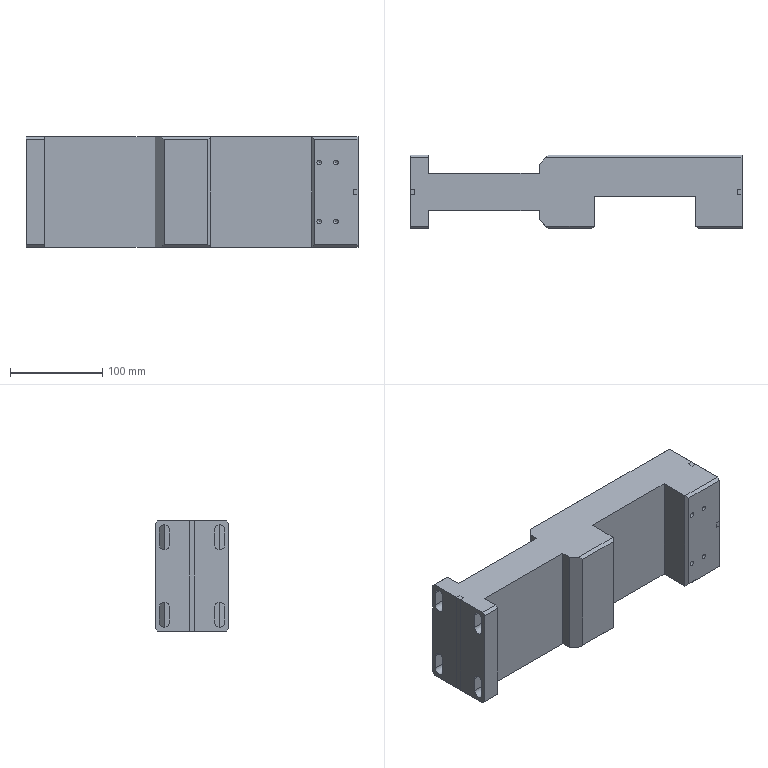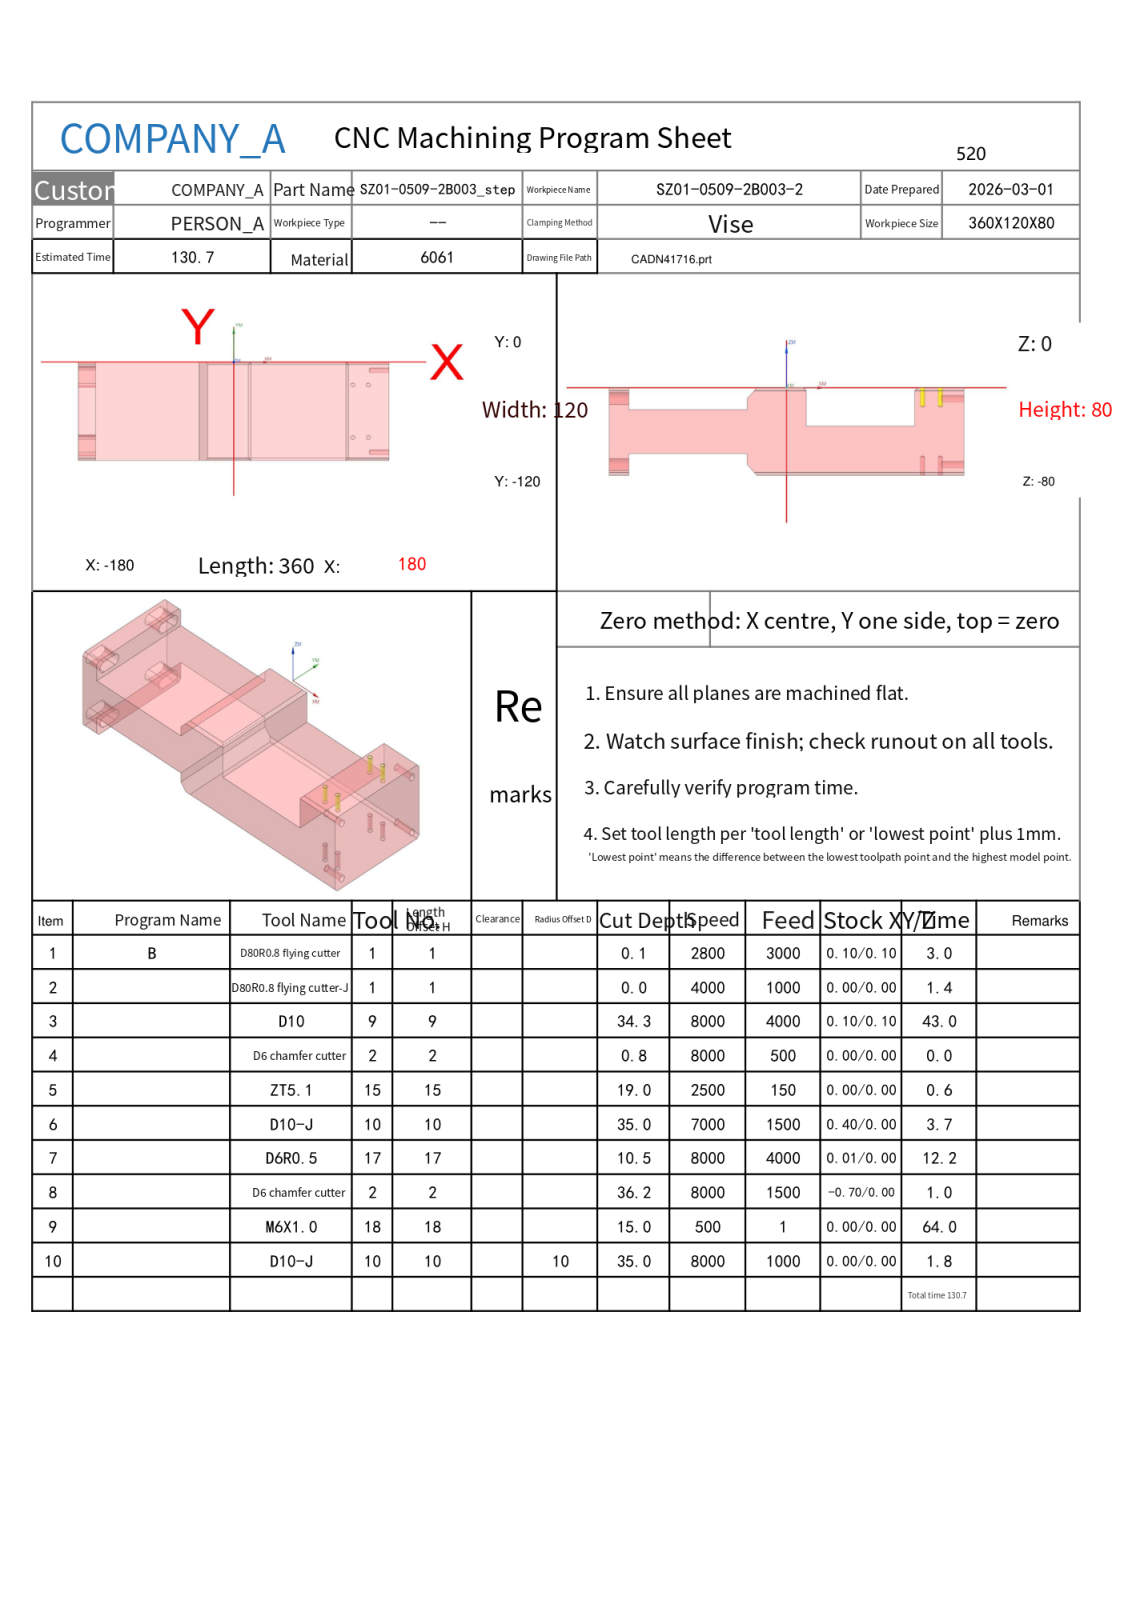NC program | NX | posted by the shop | part box 360 x 80 x 120 mm
Lines 12102 to 12457 of 12457:
N8 T02 M06
(D6 chamfer cutter  D=6. R=0. H=02 ce=0.00 di=0.00)
G00 G90 G54 X-180.99 Y-117.792 M03 S6500
G43 H02 Z50.
M08
Z.13
G01 Z-1.2 F1500.
G03 X-180.915 Y-117.452 I-1.907 J.601
G01 X-180.905 Y-117.398
X-180.928 Y-117.349
X-180.966 Y-117.259
X-181. Y-117.
Y-3.
X-180.966 Y-2.741
X-180.928 Y-2.651
X-180.905 Y-2.602
X-180.915 Y-2.548
G03 X-180.99 Y-2.208 I-1.983 J-.261
G01 Z.13
G00 Z10.
X-159.01
Z.13
G01 Z-1.2
G03 X-159.085 Y-2.548 I1.907 J-.601
G01 X-159.095 Y-2.602
X-159.072 Y-2.651
X-159.034 Y-2.741
X-159. Y-3.
Y-60.
Y-117.
X-159.034 Y-117.259
X-159.072 Y-117.349
X-159.095 Y-117.398
X-159.085 Y-117.452
G03 X-159.01 Y-117.792 I1.983 J.261
G01 Z.13
G00 Z10.
X180.99 Y-2.208
Z.13
G01 Z-1.2
G03 X180.915 Y-2.548 I1.907 J-.601
G01 X180.905 Y-2.602
X180.928 Y-2.651
X180.966 Y-2.741
X181. Y-3.
Y-117.
X180.966 Y-117.259
X180.928 Y-117.349
X180.905 Y-117.398
X180.915 Y-117.452
G03 X180.99 Y-117.792 I1.983 J.261
G01 Z.13
G00 Z10.
X137.593 Y-29.315
Z.284
G01 Z-1.2
G03 X137.898 Y-29.484 I1.118 J1.658
G01 X137.946 Y-29.509
X138. Y-29.5
G03 X139.5 Y-28. I0.0 J1.5
X138. Y-26.5 I-1.5 J0.0
X136.5 Y-28. I0.0 J-1.5
X138. Y-29.5 I1.5 J0.0
G01 X138.054 Y-29.509
X138.102 Y-29.484
G03 X138.407 Y-29.315 I-.813 J1.827
G01 Z.284
G00 Z10.
X155.593
Z.284
G01 Z-1.2
G03 X155.898 Y-29.484 I1.118 J1.658
G01 X155.946 Y-29.509
X156. Y-29.5
G03 X157.5 Y-28. I0.0 J1.5
X156. Y-26.5 I-1.5 J0.0
X154.5 Y-28. I0.0 J-1.5
X156. Y-29.5 I1.5 J0.0
G01 X156.054 Y-29.509
X156.102 Y-29.484
G03 X156.407 Y-29.315 I-.813 J1.827
G01 Z.284
G00 Z10.
X155.593 Y-93.315
Z.284
G01 Z-1.2
G03 X155.898 Y-93.484 I1.118 J1.658
G01 X155.946 Y-93.509
X156. Y-93.5
G03 X157.5 Y-92. I0.0 J1.5
X156. Y-90.5 I-1.5 J0.0
X154.5 Y-92. I0.0 J-1.5
X156. Y-93.5 I1.5 J0.0
G01 X156.054 Y-93.509
X156.102 Y-93.484
G03 X156.407 Y-93.315 I-.813 J1.827
G01 Z.284
G00 Z10.
X137.593
Z.284
G01 Z-1.2
G03 X137.898 Y-93.484 I1.118 J1.658
G01 X137.946 Y-93.509
X138. Y-93.5
G03 X139.5 Y-92. I0.0 J1.5
X138. Y-90.5 I-1.5 J0.0
X136.5 Y-92. I0.0 J-1.5
X138. Y-93.5 I1.5 J0.0
G01 X138.054 Y-93.509
X138.102 Y-93.484
G03 X138.407 Y-93.315 I-.813 J1.827
G01 Z.284
G00 Z10.
X-43.019 Y-121.068
Z-11.096
G01 Z-21.2
X-43.105 Y-121.008
X-43.135 Y-121.
X-156.865
X-156.895 Y-121.008
X-156.981 Y-121.068
Z-3.291
G00 Z10.
Y1.068
Z-3.291
G01 Z-21.2
X-156.895 Y1.008
X-156.865 Y1.
X-43.135
X-43.105 Y1.008
X-43.019 Y1.068
Z-11.096
G00 Z10.
X23.038 Y1.045
Z-4.379
G01 Z-36.2
X23.095 Y1.005
X23.115 Y1.
X126.885
X126.905 Y1.005
X126.962 Y1.045
Z-4.379
G00 Z10.
Y-121.045
Z-4.379
G01 Z-36.2
X126.905 Y-121.005
X126.885 Y-121.
X23.115
X23.095 Y-121.005
X23.038 Y-121.045
Z-4.379
G00 Z50.
G00 G90 X155.13 Y-28.232 M03 S8000
Z50.
Z-.8
G01 Z-1.3 F600.
X154.5 Y-28.4
G03 X156. Y-29.9 I1.5 J0.0
X157.9 Y-28. I0.0 J1.9
X156. Y-26.1 I-1.9 J0.0
X154.1 Y-28. I0.0 J-1.9
X156. Y-29.9 I1.9 J0.0
X157.5 Y-28.4 I0.0 J1.5
G01 X156.87 Y-28.232
Z-.8
G00 Z50.
X137.13
Z-.8
G01 Z-1.3
X136.5 Y-28.4
G03 X138. Y-29.9 I1.5 J0.0
X139.9 Y-28. I0.0 J1.9
X138. Y-26.1 I-1.9 J0.0
X136.1 Y-28. I0.0 J-1.9
X138. Y-29.9 I1.9 J0.0
X139.5 Y-28.4 I0.0 J1.5
G01 X138.87 Y-28.232
Z-.8
G00 Z50.
X137.13 Y-92.232
Z-.8
G01 Z-1.3
X136.5 Y-92.4
G03 X138. Y-93.9 I1.5 J0.0
X139.9 Y-92. I0.0 J1.9
X138. Y-90.1 I-1.9 J0.0
X136.1 Y-92. I0.0 J-1.9
X138. Y-93.9 I1.9 J0.0
X139.5 Y-92.4 I0.0 J1.5
G01 X138.87 Y-92.232
Z-.8
G00 Z50.
X155.13
Z-.8
G01 Z-1.3
X154.5 Y-92.4
G03 X156. Y-93.9 I1.5 J0.0
X157.9 Y-92. I0.0 J1.9
X156. Y-90.1 I-1.9 J0.0
X154.1 Y-92. I0.0 J-1.9
X156. Y-93.9 I1.9 J0.0
X157.5 Y-92.4 I0.0 J1.5
G01 X156.87 Y-92.232
Z-.8
G00 Z50.
G91 G28 Z0.0
M05
M09
G91 G28 Z0.0
M01
N9 T18 M06
(M6X1.0 D=5. DR_a=180 H=18)
G00 G90 G54 X138. Y-28. M03 S500
G43 H18 Z50.
M08
G95
G98 G84 X138. Y-28. Z-15. R1. F1. Q3.
X156.
Y-92.
X138.
G80
G94
G00 Z50.
G91 G28 Z0.0
M05
M09
G91 G28 Z0.0
M01
N10 T10 M06
(D10-J  D=10. R=0. H=10 ce=0.00 di=0.00)
G00 G90 G54 X-47.199 Y-127. M03 S8000
G43 H10 Z14.5
M08
Z-9.
G01 Z-10. F1000.
G41 D10
X-46.999
G03 X-45. Y-125. I-.001 J2.
G01 Y5.
G03 X-46.999 Y7. I-2. J0.0
G01 G40 X-47.199
Z-9.
G00 X-152.801
G01 Z-10.
G41 D10
X-153.001
G03 X-155. Y5. I.001 J-2.
G01 Y-125.
G03 X-153.001 Y-127. I2. J0.0
G01 G40 X-152.801
Z-9.
G00 X-47.199
Z-19.
G01 Z-20.
G41 D10
X-46.999
G03 X-45. Y-125. I-.001 J2.
G01 Y5.
G03 X-46.999 Y7. I-2. J0.0
G01 G40 X-47.199
Z-19.
G00 X-152.801
G01 Z-20.
G41 D10
X-153.001
G03 X-155. Y5. I.001 J-2.
G01 Y-125.
G03 X-153.001 Y-127. I2. J0.0
G01 G40 X-152.801
Z-19.
G00 Z14.5
G00 G90 X122.801 Y-127. M03 S8000
Z14.5
Z-7.75
G01 Z-8.75 F1000.
G41 D10
X123.001
G03 X125. Y-125. I-.001 J2.
G01 Y5.
G03 X123.001 Y7. I-2. J0.0
G01 G40 X122.801
Z-7.75
G00 X27.199
G01 Z-8.75
G41 D10
X26.999
G03 X25. Y5. I.001 J-2.
G01 Y-125.
G03 X26.999 Y-127. I2. J0.0
G01 G40 X27.199
Z-7.75
G00 X122.801
Z-16.5
G01 Z-17.5
G41 D10
X123.001
G03 X125. Y-125. I-.001 J2.
G01 Y5.
G03 X123.001 Y7. I-2. J0.0
G01 G40 X122.801
Z-16.5
G00 X27.199
G01 Z-17.5
G41 D10
X26.999
G03 X25. Y5. I.001 J-2.
G01 Y-125.
G03 X26.999 Y-127. I2. J0.0
G01 G40 X27.199
Z-16.5
G00 X122.801
Z-25.25
G01 Z-26.25
G41 D10
X123.001
G03 X125. Y-125. I-.001 J2.
G01 Y5.
G03 X123.001 Y7. I-2. J0.0
G01 G40 X122.801
Z-25.25
G00 X27.199
G01 Z-26.25
G41 D10
X26.999
G03 X25. Y5. I.001 J-2.
G01 Y-125.
G03 X26.999 Y-127. I2. J0.0
G01 G40 X27.199
Z-25.25
G00 X122.801
Z-34.
G01 Z-35.
G41 D10
X123.001
G03 X125. Y-125. I-.001 J2.
G01 Y5.
G03 X123.001 Y7. I-2. J0.0
G01 G40 X122.801
Z-34.
G00 X27.199
G01 Z-35.
G41 D10
X26.999
G03 X25. Y5. I.001 J-2.
G01 Y-125.
G03 X26.999 Y-127. I2. J0.0
G01 G40 X27.199
Z-34.
G00 Z14.5
M05
M09
G91 G28 Z0.0
G91 G28 Y0.0
M30
%